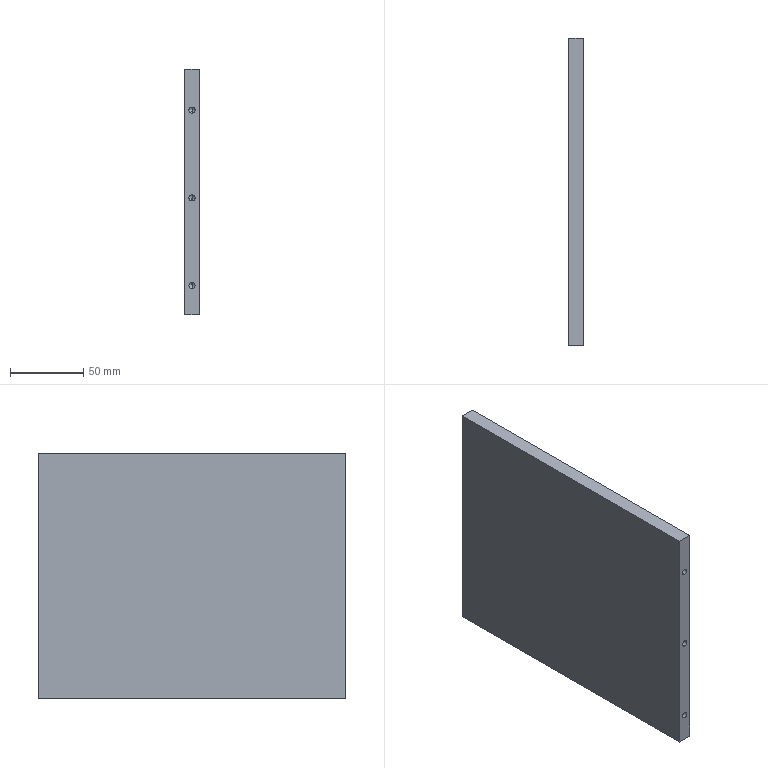Part | STEP file | 03-02 Loading-unloading side plate 2 | 1 solid | 30 faces | box 10 x 210 x 168 mm | volume 351568 mm3 | cylinder 12 | cone 12 | plane 6 | commonest cylinder face diameters 4.2 x12